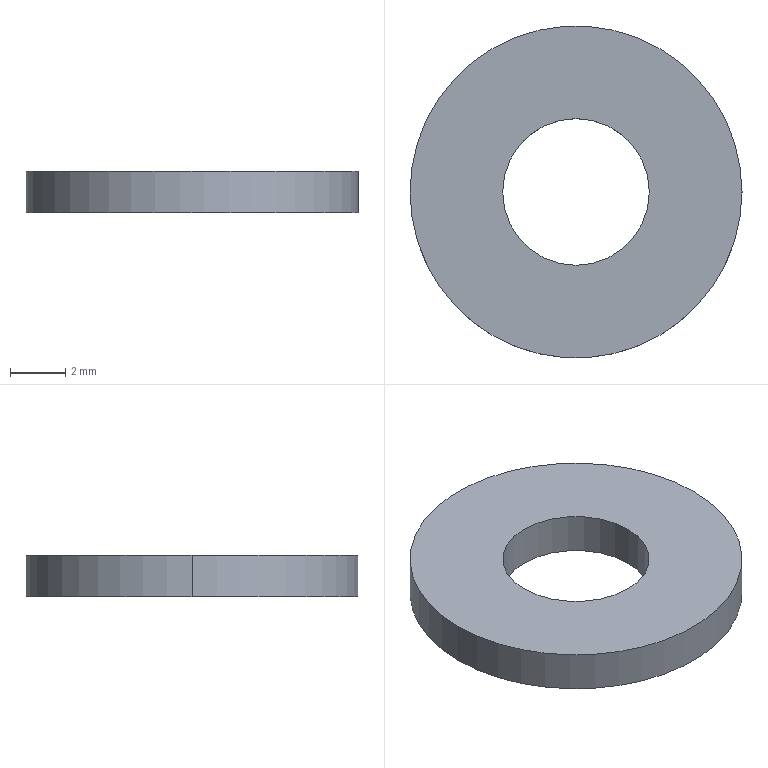Part | SolidWorks | features BaseBody 1 | 1 solid | 26 faces | box 12.059 x 12.059 x 1.507 mm | volume 122.712 mm3 | plane 14 | cylinder 12 | commonest cylinder face diameters 7.336 x4 10.049 x4 5.326 x2 12.059 x2
STEP:
#1=CARTESIAN_POINT('',(19.606,26.12,-12.71));
#2=VERTEX_POINT('',#1);
#3=CARTESIAN_POINT('',(7.547,26.12,-12.71));
#4=VERTEX_POINT('',#3);
#5=CARTESIAN_POINT('',(13.577,26.12,-12.71));
#6=DIRECTION('',(0.,0.,1.));
#7=DIRECTION('',(-1.,0.,0.));
#8=AXIS2_PLACEMENT_3D('',#5,#6,#7);
#9=CIRCLE('',#8,6.03);
#10=EDGE_CURVE('',#2,#4,#9,.T.);
#11=ORIENTED_EDGE('',*,*,#10,.F.);
#12=CARTESIAN_POINT('',(19.606,26.12,-14.217));
#13=VERTEX_POINT('',#12);
#14=CARTESIAN_POINT('',(19.606,26.12,-12.71));
#15=DIRECTION('',(0.,0.,-1.));
#16=VECTOR('',#15,1000.);
#17=LINE('',#14,#16);
#18=EDGE_CURVE('',#2,#13,#17,.T.);
#19=ORIENTED_EDGE('',*,*,#18,.T.);
#20=CARTESIAN_POINT('',(7.547,26.12,-14.217));
#21=VERTEX_POINT('',#20);
#22=CARTESIAN_POINT('',(13.577,26.12,-14.217));
#23=DIRECTION('',(0.,0.,1.));
#24=DIRECTION('',(-1.,0.,0.));
#25=AXIS2_PLACEMENT_3D('',#22,#23,#24);
#26=CIRCLE('',#25,6.03);
#27=EDGE_CURVE('',#13,#21,#26,.T.);
#28=ORIENTED_EDGE('',*,*,#27,.T.);
#29=CARTESIAN_POINT('',(7.547,26.12,-12.71));
#30=DIRECTION('',(0.,0.,-1.));
#31=VECTOR('',#30,1000.);
#32=LINE('',#29,#31);
#33=EDGE_CURVE('',#4,#21,#32,.T.);
#34=ORIENTED_EDGE('',*,*,#33,.F.);
#35=EDGE_LOOP('',(#11,#19,#28,#34));
#36=FACE_OUTER_BOUND('',#35,.T.);
#37=CARTESIAN_POINT('',(13.577,26.12,-12.71));
#38=DIRECTION('',(0.,0.,-1.));
#39=DIRECTION('',(-1.,0.,0.));
#40=AXIS2_PLACEMENT_3D('',#37,#38,#39);
#41=CYLINDRICAL_SURFACE('',#40,6.03);
#42=ADVANCED_FACE('',(#36),#41,.T.);
#43=CARTESIAN_POINT('',(16.24,26.12,-12.71));
#44=VERTEX_POINT('',#43);
#45=CARTESIAN_POINT('',(10.914,26.12,-12.71));
#46=VERTEX_POINT('',#45);
#47=CARTESIAN_POINT('',(13.577,26.12,-12.71));
#48=DIRECTION('',(0.,0.,-1.));
#49=DIRECTION('',(-1.,0.,0.));
#50=AXIS2_PLACEMENT_3D('',#47,#48,#49);
#51=CIRCLE('',#50,2.663);
#52=EDGE_CURVE('',#44,#46,#51,.T.);
#53=ORIENTED_EDGE('',*,*,#52,.F.);
#54=CARTESIAN_POINT('',(16.24,26.12,-14.217));
#55=VERTEX_POINT('',#54);
#56=CARTESIAN_POINT('',(16.24,26.12,-12.71));
#57=DIRECTION('',(0.,0.,-1.));
#58=VECTOR('',#57,1000.);
#59=LINE('',#56,#58);
#60=EDGE_CURVE('',#44,#55,#59,.T.);
#61=ORIENTED_EDGE('',*,*,#60,.T.);
#62=CARTESIAN_POINT('',(10.914,26.12,-14.217));
#63=VERTEX_POINT('',#62);
#64=CARTESIAN_POINT('',(13.577,26.12,-14.217));
#65=DIRECTION('',(0.,0.,1.));
#66=DIRECTION('',(-1.,0.,0.));
#67=AXIS2_PLACEMENT_3D('',#64,#65,#66);
#68=CIRCLE('',#67,2.663);
#69=EDGE_CURVE('',#63,#55,#68,.T.);
#70=ORIENTED_EDGE('',*,*,#69,.F.);
#71=CARTESIAN_POINT('',(10.914,26.12,-12.71));
#72=DIRECTION('',(0.,0.,-1.));
#73=VECTOR('',#72,1000.);
#74=LINE('',#71,#73);
#75=EDGE_CURVE('',#46,#63,#74,.T.);
#76=ORIENTED_EDGE('',*,*,#75,.F.);
#77=EDGE_LOOP('',(#53,#61,#70,#76));
#78=FACE_OUTER_BOUND('',#77,.T.);
#79=CARTESIAN_POINT('',(13.577,26.12,-12.71));
#80=DIRECTION('',(0.,0.,-1.));
#81=DIRECTION('',(-1.,0.,0.));
#82=AXIS2_PLACEMENT_3D('',#79,#80,#81);
#83=CYLINDRICAL_SURFACE('',#82,2.663);
#84=ADVANCED_FACE('',(#78),#83,.F.);
#85=CARTESIAN_POINT('',(13.577,26.12,-12.71));
#86=DIRECTION('',(0.,0.,1.));
#87=DIRECTION('',(-1.,0.,0.));
#88=AXIS2_PLACEMENT_3D('',#85,#86,#87);
#89=CIRCLE('',#88,6.03);
#90=EDGE_CURVE('',#4,#2,#89,.T.);
#91=ORIENTED_EDGE('',*,*,#90,.T.);
#92=ORIENTED_EDGE('',*,*,#10,.T.);
#93=EDGE_LOOP('',(#91,#92));
#94=FACE_OUTER_BOUND('',#93,.T.);
#95=CARTESIAN_POINT('',(13.577,26.12,-12.71));
#96=DIRECTION('',(0.,0.,-1.));
#97=DIRECTION('',(-1.,0.,0.));
#98=AXIS2_PLACEMENT_3D('',#95,#96,#97);
#99=CIRCLE('',#98,2.663);
#100=EDGE_CURVE('',#46,#44,#99,.T.);
#101=ORIENTED_EDGE('',*,*,#100,.T.);
#102=ORIENTED_EDGE('',*,*,#52,.T.);
#103=EDGE_LOOP('',(#101,#102));
#104=FACE_BOUND('',#103,.T.);
#105=CARTESIAN_POINT('',(13.577,26.12,-12.71));
#106=DIRECTION('',(0.,0.,1.));
#107=DIRECTION('',(1.,0.,0.));
#108=AXIS2_PLACEMENT_3D('',#105,#106,#107);
#109=PLANE('',#108);
#110=ADVANCED_FACE('',(#94,#104),#109,.T.);
#111=ORIENTED_EDGE('',*,*,#18,.F.);
#112=ORIENTED_EDGE('',*,*,#90,.F.);
#113=ORIENTED_EDGE('',*,*,#33,.T.);
#114=CARTESIAN_POINT('',(13.577,26.12,-14.217));
#115=DIRECTION('',(0.,0.,1.));
#116=DIRECTION('',(-1.,0.,0.));
#117=AXIS2_PLACEMENT_3D('',#114,#115,#116);
#118=CIRCLE('',#117,6.03);
#119=EDGE_CURVE('',#21,#13,#118,.T.);
#120=ORIENTED_EDGE('',*,*,#119,.T.);
#121=EDGE_LOOP('',(#111,#112,#113,#120));
#122=FACE_OUTER_BOUND('',#121,.T.);
#123=CARTESIAN_POINT('',(13.577,26.12,-12.71));
#124=DIRECTION('',(0.,0.,-1.));
#125=DIRECTION('',(-1.,0.,0.));
#126=AXIS2_PLACEMENT_3D('',#123,#124,#125);
#127=CYLINDRICAL_SURFACE('',#126,6.03);
#128=ADVANCED_FACE('',(#122),#127,.T.);
#129=ORIENTED_EDGE('',*,*,#60,.F.);
#130=ORIENTED_EDGE('',*,*,#100,.F.);
#131=ORIENTED_EDGE('',*,*,#75,.T.);
#132=CARTESIAN_POINT('',(13.577,26.12,-14.217));
#133=DIRECTION('',(0.,0.,1.));
#134=DIRECTION('',(-1.,0.,0.));
#135=AXIS2_PLACEMENT_3D('',#132,#133,#134);
#136=CIRCLE('',#135,2.663);
#137=EDGE_CURVE('',#55,#63,#136,.T.);
#138=ORIENTED_EDGE('',*,*,#137,.F.);
#139=EDGE_LOOP('',(#129,#130,#131,#138));
#140=FACE_OUTER_BOUND('',#139,.T.);
#141=CARTESIAN_POINT('',(13.577,26.12,-12.71));
#142=DIRECTION('',(0.,0.,-1.));
#143=DIRECTION('',(-1.,0.,0.));
#144=AXIS2_PLACEMENT_3D('',#141,#142,#143);
#145=CYLINDRICAL_SURFACE('',#144,2.663);
#146=ADVANCED_FACE('',(#140),#145,.F.);
#147=CARTESIAN_POINT('',(18.576,25.618,-14.217));
#148=VERTEX_POINT('',#147);
#149=CARTESIAN_POINT('',(14.079,21.121,-14.217));
#150=VERTEX_POINT('',#149);
#151=CARTESIAN_POINT('',(13.577,26.12,-14.217));
#152=DIRECTION('',(0.,0.,-1.));
#153=DIRECTION('',(-1.,0.,0.));
#154=AXIS2_PLACEMENT_3D('',#151,#152,#153);
#155=CIRCLE('',#154,5.025);
#156=EDGE_CURVE('',#148,#150,#155,.T.);
#157=ORIENTED_EDGE('',*,*,#156,.F.);
#158=CARTESIAN_POINT('',(17.21,25.618,-14.217));
#159=VERTEX_POINT('',#158);
#160=CARTESIAN_POINT('',(13.577,25.618,-14.217));
#161=DIRECTION('',(1.,0.,0.));
#162=VECTOR('',#161,1000.);
#163=LINE('',#160,#162);
#164=EDGE_CURVE('',#159,#148,#163,.T.);
#165=ORIENTED_EDGE('',*,*,#164,.F.);
#166=CARTESIAN_POINT('',(14.079,22.487,-14.217));
#167=VERTEX_POINT('',#166);
#168=CARTESIAN_POINT('',(13.577,26.12,-14.217));
#169=DIRECTION('',(0.,0.,1.));
#170=DIRECTION('',(-1.,0.,0.));
#171=AXIS2_PLACEMENT_3D('',#168,#169,#170);
#172=CIRCLE('',#171,3.668);
#173=EDGE_CURVE('',#167,#159,#172,.T.);
#174=ORIENTED_EDGE('',*,*,#173,.F.);
#175=CARTESIAN_POINT('',(14.079,26.12,-14.217));
#176=DIRECTION('',(0.,1.,0.));
#177=VECTOR('',#176,1000.);
#178=LINE('',#175,#177);
#179=EDGE_CURVE('',#150,#167,#178,.T.);
#180=ORIENTED_EDGE('',*,*,#179,.F.);
#181=EDGE_LOOP('',(#157,#165,#174,#180));
#182=FACE_BOUND('',#181,.T.);
#183=CARTESIAN_POINT('',(13.074,22.487,-14.217));
#184=VERTEX_POINT('',#183);
#185=CARTESIAN_POINT('',(13.074,21.121,-14.217));
#186=VERTEX_POINT('',#185);
#187=CARTESIAN_POINT('',(13.074,26.12,-14.217));
#188=DIRECTION('',(0.,-1.,0.));
#189=VECTOR('',#188,1000.);
#190=LINE('',#187,#189);
#191=EDGE_CURVE('',#184,#186,#190,.T.);
#192=ORIENTED_EDGE('',*,*,#191,.F.);
#193=CARTESIAN_POINT('',(9.943,25.618,-14.217));
#194=VERTEX_POINT('',#193);
#195=CARTESIAN_POINT('',(13.577,26.12,-14.217));
#196=DIRECTION('',(0.,0.,1.));
#197=DIRECTION('',(-1.,0.,0.));
#198=AXIS2_PLACEMENT_3D('',#195,#196,#197);
#199=CIRCLE('',#198,3.668);
#200=EDGE_CURVE('',#194,#184,#199,.T.);
#201=ORIENTED_EDGE('',*,*,#200,.F.);
#202=CARTESIAN_POINT('',(8.577,25.618,-14.217));
#203=VERTEX_POINT('',#202);
#204=CARTESIAN_POINT('',(13.577,25.618,-14.217));
#205=DIRECTION('',(1.,0.,0.));
#206=VECTOR('',#205,1000.);
#207=LINE('',#204,#206);
#208=EDGE_CURVE('',#203,#194,#207,.T.);
#209=ORIENTED_EDGE('',*,*,#208,.F.);
#210=CARTESIAN_POINT('',(13.577,26.12,-14.217));
#211=DIRECTION('',(0.,0.,-1.));
#212=DIRECTION('',(-1.,0.,0.));
#213=AXIS2_PLACEMENT_3D('',#210,#211,#212);
#214=CIRCLE('',#213,5.025);
#215=EDGE_CURVE('',#186,#203,#214,.T.);
#216=ORIENTED_EDGE('',*,*,#215,.F.);
#217=EDGE_LOOP('',(#192,#201,#209,#216));
#218=FACE_BOUND('',#217,.T.);
#219=ORIENTED_EDGE('',*,*,#119,.F.);
#220=ORIENTED_EDGE('',*,*,#27,.F.);
#221=EDGE_LOOP('',(#219,#220));
#222=FACE_OUTER_BOUND('',#221,.T.);
#223=CARTESIAN_POINT('',(14.079,29.753,-14.217));
#224=VERTEX_POINT('',#223);
#225=CARTESIAN_POINT('',(14.079,31.119,-14.217));
#226=VERTEX_POINT('',#225);
#227=CARTESIAN_POINT('',(14.079,26.12,-14.217));
#228=DIRECTION('',(0.,1.,0.));
#229=VECTOR('',#228,1000.);
#230=LINE('',#227,#229);
#231=EDGE_CURVE('',#224,#226,#230,.T.);
#232=ORIENTED_EDGE('',*,*,#231,.F.);
#233=CARTESIAN_POINT('',(17.21,26.622,-14.217));
#234=VERTEX_POINT('',#233);
#235=CARTESIAN_POINT('',(13.577,26.12,-14.217));
#236=DIRECTION('',(0.,0.,1.));
#237=DIRECTION('',(-1.,0.,0.));
#238=AXIS2_PLACEMENT_3D('',#235,#236,#237);
#239=CIRCLE('',#238,3.668);
#240=EDGE_CURVE('',#234,#224,#239,.T.);
#241=ORIENTED_EDGE('',*,*,#240,.F.);
#242=CARTESIAN_POINT('',(18.576,26.622,-14.217));
#243=VERTEX_POINT('',#242);
#244=CARTESIAN_POINT('',(13.577,26.622,-14.217));
#245=DIRECTION('',(-1.,0.,0.));
#246=VECTOR('',#245,1000.);
#247=LINE('',#244,#246);
#248=EDGE_CURVE('',#243,#234,#247,.T.);
#249=ORIENTED_EDGE('',*,*,#248,.F.);
#250=CARTESIAN_POINT('',(13.577,26.12,-14.217));
#251=DIRECTION('',(0.,0.,-1.));
#252=DIRECTION('',(-1.,0.,0.));
#253=AXIS2_PLACEMENT_3D('',#250,#251,#252);
#254=CIRCLE('',#253,5.025);
#255=EDGE_CURVE('',#226,#243,#254,.T.);
#256=ORIENTED_EDGE('',*,*,#255,.F.);
#257=EDGE_LOOP('',(#232,#241,#249,#256));
#258=FACE_BOUND('',#257,.T.);
#259=ORIENTED_EDGE('',*,*,#69,.T.);
#260=ORIENTED_EDGE('',*,*,#137,.T.);
#261=EDGE_LOOP('',(#259,#260));
#262=FACE_BOUND('',#261,.T.);
#263=CARTESIAN_POINT('',(8.577,26.622,-14.217));
#264=VERTEX_POINT('',#263);
#265=CARTESIAN_POINT('',(13.074,31.119,-14.217));
#266=VERTEX_POINT('',#265);
#267=CARTESIAN_POINT('',(13.577,26.12,-14.217));
#268=DIRECTION('',(0.,0.,-1.));
#269=DIRECTION('',(-1.,0.,0.));
#270=AXIS2_PLACEMENT_3D('',#267,#268,#269);
#271=CIRCLE('',#270,5.025);
#272=EDGE_CURVE('',#264,#266,#271,.T.);
#273=ORIENTED_EDGE('',*,*,#272,.F.);
#274=CARTESIAN_POINT('',(9.943,26.622,-14.217));
#275=VERTEX_POINT('',#274);
#276=CARTESIAN_POINT('',(13.577,26.622,-14.217));
#277=DIRECTION('',(-1.,0.,0.));
#278=VECTOR('',#277,1000.);
#279=LINE('',#276,#278);
#280=EDGE_CURVE('',#275,#264,#279,.T.);
#281=ORIENTED_EDGE('',*,*,#280,.F.);
#282=CARTESIAN_POINT('',(13.074,29.753,-14.217));
#283=VERTEX_POINT('',#282);
#284=CARTESIAN_POINT('',(13.577,26.12,-14.217));
#285=DIRECTION('',(0.,0.,1.));
#286=DIRECTION('',(-1.,0.,0.));
#287=AXIS2_PLACEMENT_3D('',#284,#285,#286);
#288=CIRCLE('',#287,3.668);
#289=EDGE_CURVE('',#283,#275,#288,.T.);
#290=ORIENTED_EDGE('',*,*,#289,.F.);
#291=CARTESIAN_POINT('',(13.074,26.12,-14.217));
#292=DIRECTION('',(0.,-1.,0.));
#293=VECTOR('',#292,1000.);
#294=LINE('',#291,#293);
#295=EDGE_CURVE('',#266,#283,#294,.T.);
#296=ORIENTED_EDGE('',*,*,#295,.F.);
#297=EDGE_LOOP('',(#273,#281,#290,#296));
#298=FACE_BOUND('',#297,.T.);
#299=CARTESIAN_POINT('',(13.577,26.12,-14.217));
#300=DIRECTION('',(0.,0.,1.));
#301=DIRECTION('',(1.,0.,0.));
#302=AXIS2_PLACEMENT_3D('',#299,#300,#301);
#303=PLANE('',#302);
#304=ADVANCED_FACE('',(#182,#218,#222,#258,#262,#298),#303,.F.);
#305=CARTESIAN_POINT('',(14.079,22.487,-13.715));
#306=VERTEX_POINT('',#305);
#307=CARTESIAN_POINT('',(14.079,21.121,-13.715));
#308=VERTEX_POINT('',#307);
#309=CARTESIAN_POINT('',(14.079,26.12,-13.715));
#310=DIRECTION('',(0.,-1.,0.));
#311=VECTOR('',#310,1000.);
#312=LINE('',#309,#311);
#313=EDGE_CURVE('',#306,#308,#312,.T.);
#314=ORIENTED_EDGE('',*,*,#313,.T.);
#315=CARTESIAN_POINT('',(14.079,21.121,-14.217));
#316=DIRECTION('',(0.,0.,1.));
#317=VECTOR('',#316,1000.);
#318=LINE('',#315,#317);
#319=EDGE_CURVE('',#150,#308,#318,.T.);
#320=ORIENTED_EDGE('',*,*,#319,.F.);
#321=ORIENTED_EDGE('',*,*,#179,.T.);
#322=CARTESIAN_POINT('',(14.079,22.487,-14.217));
#323=DIRECTION('',(0.,0.,-1.));
#324=VECTOR('',#323,1000.);
#325=LINE('',#322,#324);
#326=EDGE_CURVE('',#306,#167,#325,.T.);
#327=ORIENTED_EDGE('',*,*,#326,.F.);
#328=EDGE_LOOP('',(#314,#320,#321,#327));
#329=FACE_OUTER_BOUND('',#328,.T.);
#330=CARTESIAN_POINT('',(14.079,22.882,-14.217));
#331=DIRECTION('',(-1.,0.,0.));
#332=DIRECTION('',(0.,-1.,0.));
#333=AXIS2_PLACEMENT_3D('',#330,#331,#332);
#334=PLANE('',#333);
#335=ADVANCED_FACE('',(#329),#334,.F.);
#336=CARTESIAN_POINT('',(18.576,25.618,-13.715));
#337=VERTEX_POINT('',#336);
#338=CARTESIAN_POINT('',(18.576,25.618,-12.71));
#339=DIRECTION('',(0.,0.,1.));
#340=VECTOR('',#339,1000.);
#341=LINE('',#338,#340);
#342=EDGE_CURVE('',#148,#337,#341,.T.);
#343=ORIENTED_EDGE('',*,*,#342,.F.);
#344=ORIENTED_EDGE('',*,*,#156,.T.);
#345=ORIENTED_EDGE('',*,*,#319,.T.);
#346=CARTESIAN_POINT('',(13.577,26.12,-13.715));
#347=DIRECTION('',(0.,0.,-1.));
#348=DIRECTION('',(-1.,0.,0.));
#349=AXIS2_PLACEMENT_3D('',#346,#347,#348);
#350=CIRCLE('',#349,5.025);
#351=EDGE_CURVE('',#337,#308,#350,.T.);
#352=ORIENTED_EDGE('',*,*,#351,.F.);
#353=EDGE_LOOP('',(#343,#344,#345,#352));
#354=FACE_OUTER_BOUND('',#353,.T.);
#355=CARTESIAN_POINT('',(13.577,26.12,-12.71));
#356=DIRECTION('',(0.,0.,-1.));
#357=DIRECTION('',(-1.,0.,0.));
#358=AXIS2_PLACEMENT_3D('',#355,#356,#357);
#359=CYLINDRICAL_SURFACE('',#358,5.025);
#360=ADVANCED_FACE('',(#354),#359,.F.);
#361=CARTESIAN_POINT('',(17.21,25.618,-13.715));
#362=VERTEX_POINT('',#361);
#363=CARTESIAN_POINT('',(16.815,25.618,-13.715));
#364=DIRECTION('',(-1.,0.,0.));
#365=VECTOR('',#364,1000.);
#366=LINE('',#363,#365);
#367=EDGE_CURVE('',#337,#362,#366,.T.);
#368=ORIENTED_EDGE('',*,*,#367,.T.);
#369=CARTESIAN_POINT('',(17.21,25.618,-14.217));
#370=DIRECTION('',(0.,0.,-1.));
#371=VECTOR('',#370,1000.);
#372=LINE('',#369,#371);
#373=EDGE_CURVE('',#362,#159,#372,.T.);
#374=ORIENTED_EDGE('',*,*,#373,.T.);
#375=ORIENTED_EDGE('',*,*,#164,.T.);
#376=ORIENTED_EDGE('',*,*,#342,.T.);
#377=EDGE_LOOP('',(#368,#374,#375,#376));
#378=FACE_OUTER_BOUND('',#377,.T.);
#379=CARTESIAN_POINT('',(16.815,25.618,-14.217));
#380=DIRECTION('',(0.,-1.,0.));
#381=DIRECTION('',(1.,0.,0.));
#382=AXIS2_PLACEMENT_3D('',#379,#380,#381);
#383=PLANE('',#382);
#384=ADVANCED_FACE('',(#378),#383,.T.);
#385=ORIENTED_EDGE('',*,*,#373,.F.);
#386=CARTESIAN_POINT('',(13.577,26.12,-13.715));
#387=DIRECTION('',(0.,0.,-1.));
#388=DIRECTION('',(-1.,0.,0.));
#389=AXIS2_PLACEMENT_3D('',#386,#387,#388);
#390=CIRCLE('',#389,3.668);
#391=EDGE_CURVE('',#362,#306,#390,.T.);
#392=ORIENTED_EDGE('',*,*,#391,.T.);
#393=ORIENTED_EDGE('',*,*,#326,.T.);
#394=ORIENTED_EDGE('',*,*,#173,.T.);
#395=EDGE_LOOP('',(#385,#392,#393,#394));
#396=FACE_OUTER_BOUND('',#395,.T.);
#397=CARTESIAN_POINT('',(13.577,26.12,-12.71));
#398=DIRECTION('',(0.,0.,-1.));
#399=DIRECTION('',(-1.,0.,0.));
#400=AXIS2_PLACEMENT_3D('',#397,#398,#399);
#401=CYLINDRICAL_SURFACE('',#400,3.668);
#402=ADVANCED_FACE('',(#396),#401,.T.);
#403=CARTESIAN_POINT('',(13.074,21.121,-13.715));
#404=VERTEX_POINT('',#403);
#405=CARTESIAN_POINT('',(13.074,21.121,-12.71));
#406=DIRECTION('',(0.,0.,1.));
#407=VECTOR('',#406,1000.);
#408=LINE('',#405,#407);
#409=EDGE_CURVE('',#186,#404,#408,.T.);
#410=ORIENTED_EDGE('',*,*,#409,.F.);
#411=ORIENTED_EDGE('',*,*,#215,.T.);
#412=CARTESIAN_POINT('',(8.577,25.618,-13.715));
#413=VERTEX_POINT('',#412);
#414=CARTESIAN_POINT('',(8.577,25.618,-12.71));
#415=DIRECTION('',(0.,0.,-1.));
#416=VECTOR('',#415,1000.);
#417=LINE('',#414,#416);
#418=EDGE_CURVE('',#413,#203,#417,.T.);
#419=ORIENTED_EDGE('',*,*,#418,.F.);
#420=CARTESIAN_POINT('',(13.577,26.12,-13.715));
#421=DIRECTION('',(0.,0.,-1.));
#422=DIRECTION('',(-1.,0.,0.));
#423=AXIS2_PLACEMENT_3D('',#420,#421,#422);
#424=CIRCLE('',#423,5.025);
#425=EDGE_CURVE('',#404,#413,#424,.T.);
#426=ORIENTED_EDGE('',*,*,#425,.F.);
#427=EDGE_LOOP('',(#410,#411,#419,#426));
#428=FACE_OUTER_BOUND('',#427,.T.);
#429=CARTESIAN_POINT('',(13.577,26.12,-12.71));
#430=DIRECTION('',(0.,0.,-1.));
#431=DIRECTION('',(-1.,0.,0.));
#432=AXIS2_PLACEMENT_3D('',#429,#430,#431);
#433=CYLINDRICAL_SURFACE('',#432,5.025);
#434=ADVANCED_FACE('',(#428),#433,.F.);
#435=CARTESIAN_POINT('',(13.074,22.487,-13.715));
#436=VERTEX_POINT('',#435);
#437=CARTESIAN_POINT('',(13.074,22.882,-13.715));
#438=DIRECTION('',(0.,1.,0.));
#439=VECTOR('',#438,1000.);
#440=LINE('',#437,#439);
#441=EDGE_CURVE('',#404,#436,#440,.T.);
#442=ORIENTED_EDGE('',*,*,#441,.T.);
#443=CARTESIAN_POINT('',(13.074,22.487,-14.217));
#444=DIRECTION('',(0.,0.,-1.));
#445=VECTOR('',#444,1000.);
#446=LINE('',#443,#445);
#447=EDGE_CURVE('',#436,#184,#446,.T.);
#448=ORIENTED_EDGE('',*,*,#447,.T.);
#449=ORIENTED_EDGE('',*,*,#191,.T.);
#450=ORIENTED_EDGE('',*,*,#409,.T.);
#451=EDGE_LOOP('',(#442,#448,#449,#450));
#452=FACE_OUTER_BOUND('',#451,.T.);
#453=CARTESIAN_POINT('',(13.074,22.882,-14.217));
#454=DIRECTION('',(-1.,0.,0.));
#455=DIRECTION('',(0.,-1.,0.));
#456=AXIS2_PLACEMENT_3D('',#453,#454,#455);
#457=PLANE('',#456);
#458=ADVANCED_FACE('',(#452),#457,.T.);
#459=ORIENTED_EDGE('',*,*,#447,.F.);
#460=CARTESIAN_POINT('',(9.943,25.618,-13.715));
#461=VERTEX_POINT('',#460);
#462=CARTESIAN_POINT('',(13.577,26.12,-13.715));
#463=DIRECTION('',(0.,0.,-1.));
#464=DIRECTION('',(-1.,0.,0.));
#465=AXIS2_PLACEMENT_3D('',#462,#463,#464);
#466=CIRCLE('',#465,3.668);
#467=EDGE_CURVE('',#436,#461,#466,.T.);
#468=ORIENTED_EDGE('',*,*,#467,.T.);
#469=CARTESIAN_POINT('',(9.943,25.618,-12.71));
#470=DIRECTION('',(0.,0.,-1.));
#471=VECTOR('',#470,1000.);
#472=LINE('',#469,#471);
#473=EDGE_CURVE('',#461,#194,#472,.T.);
#474=ORIENTED_EDGE('',*,*,#473,.T.);
#475=ORIENTED_EDGE('',*,*,#200,.T.);
#476=EDGE_LOOP('',(#459,#468,#474,#475));
#477=FACE_OUTER_BOUND('',#476,.T.);
#478=CARTESIAN_POINT('',(13.577,26.12,-12.71));
#479=DIRECTION('',(0.,0.,-1.));
#480=DIRECTION('',(-1.,0.,0.));
#481=AXIS2_PLACEMENT_3D('',#478,#479,#480);
#482=CYLINDRICAL_SURFACE('',#481,3.668);
#483=ADVANCED_FACE('',(#477),#482,.T.);
#484=CARTESIAN_POINT('',(10.338,25.618,-13.715));
#485=DIRECTION('',(1.,0.,0.));
#486=VECTOR('',#485,1000.);
#487=LINE('',#484,#486);
#488=EDGE_CURVE('',#413,#461,#487,.T.);
#489=ORIENTED_EDGE('',*,*,#488,.F.);
#490=ORIENTED_EDGE('',*,*,#418,.T.);
#491=ORIENTED_EDGE('',*,*,#208,.T.);
#492=ORIENTED_EDGE('',*,*,#473,.F.);
#493=EDGE_LOOP('',(#489,#490,#491,#492));
#494=FACE_OUTER_BOUND('',#493,.T.);
#495=CARTESIAN_POINT('',(10.338,25.618,-14.217));
#496=DIRECTION('',(0.,1.,0.));
#497=DIRECTION('',(-1.,0.,0.));
#498=AXIS2_PLACEMENT_3D('',#495,#496,#497);
#499=PLANE('',#498);
#500=ADVANCED_FACE('',(#494),#499,.F.);
#501=CARTESIAN_POINT('',(14.079,31.119,-13.715));
#502=VERTEX_POINT('',#501);
#503=CARTESIAN_POINT('',(14.079,31.119,-12.71));
#504=DIRECTION('',(0.,0.,1.));
#505=VECTOR('',#504,1000.);
#506=LINE('',#503,#505);
#507=EDGE_CURVE('',#226,#502,#506,.T.);
#508=ORIENTED_EDGE('',*,*,#507,.F.);
#509=ORIENTED_EDGE('',*,*,#255,.T.);
#510=CARTESIAN_POINT('',(18.576,26.622,-13.715));
#511=VERTEX_POINT('',#510);
#512=CARTESIAN_POINT('',(18.576,26.622,-12.71));
#513=DIRECTION('',(0.,0.,-1.));
#514=VECTOR('',#513,1000.);
#515=LINE('',#512,#514);
#516=EDGE_CURVE('',#511,#243,#515,.T.);
#517=ORIENTED_EDGE('',*,*,#516,.F.);
#518=CARTESIAN_POINT('',(13.577,26.12,-13.715));
#519=DIRECTION('',(0.,0.,-1.));
#520=DIRECTION('',(-1.,0.,0.));
#521=AXIS2_PLACEMENT_3D('',#518,#519,#520);
#522=CIRCLE('',#521,5.025);
#523=EDGE_CURVE('',#502,#511,#522,.T.);
#524=ORIENTED_EDGE('',*,*,#523,.F.);
#525=EDGE_LOOP('',(#508,#509,#517,#524));
#526=FACE_OUTER_BOUND('',#525,.T.);
#527=CARTESIAN_POINT('',(13.577,26.12,-12.71));
#528=DIRECTION('',(0.,0.,-1.));
#529=DIRECTION('',(-1.,0.,0.));
#530=AXIS2_PLACEMENT_3D('',#527,#528,#529);
#531=CYLINDRICAL_SURFACE('',#530,5.025);
#532=ADVANCED_FACE('',(#526),#531,.F.);
#533=CARTESIAN_POINT('',(14.079,29.753,-13.715));
#534=VERTEX_POINT('',#533);
#535=CARTESIAN_POINT('',(14.079,29.358,-13.715));
#536=DIRECTION('',(0.,-1.,0.));
#537=VECTOR('',#536,1000.);
#538=LINE('',#535,#537);
#539=EDGE_CURVE('',#502,#534,#538,.T.);
#540=ORIENTED_EDGE('',*,*,#539,.T.);
#541=CARTESIAN_POINT('',(14.079,29.753,-14.217));
#542=DIRECTION('',(0.,0.,-1.));
#543=VECTOR('',#542,1000.);
#544=LINE('',#541,#543);
#545=EDGE_CURVE('',#534,#224,#544,.T.);
#546=ORIENTED_EDGE('',*,*,#545,.T.);
#547=ORIENTED_EDGE('',*,*,#231,.T.);
#548=ORIENTED_EDGE('',*,*,#507,.T.);
#549=EDGE_LOOP('',(#540,#546,#547,#548));
#550=FACE_OUTER_BOUND('',#549,.T.);
#551=CARTESIAN_POINT('',(14.079,29.358,-14.217));
#552=DIRECTION('',(1.,0.,0.));
#553=DIRECTION('',(0.,1.,0.));
#554=AXIS2_PLACEMENT_3D('',#551,#552,#553);
#555=PLANE('',#554);
#556=ADVANCED_FACE('',(#550),#555,.T.);
#557=ORIENTED_EDGE('',*,*,#545,.F.);
#558=CARTESIAN_POINT('',(17.21,26.622,-13.715));
#559=VERTEX_POINT('',#558);
#560=CARTESIAN_POINT('',(13.577,26.12,-13.715));
#561=DIRECTION('',(0.,0.,-1.));
#562=DIRECTION('',(-1.,0.,0.));
#563=AXIS2_PLACEMENT_3D('',#560,#561,#562);
#564=CIRCLE('',#563,3.668);
#565=EDGE_CURVE('',#534,#559,#564,.T.);
#566=ORIENTED_EDGE('',*,*,#565,.T.);
#567=CARTESIAN_POINT('',(17.21,26.622,-12.71));
#568=DIRECTION('',(0.,0.,-1.));
#569=VECTOR('',#568,1000.);
#570=LINE('',#567,#569);
#571=EDGE_CURVE('',#559,#234,#570,.T.);
#572=ORIENTED_EDGE('',*,*,#571,.T.);
#573=ORIENTED_EDGE('',*,*,#240,.T.);
#574=EDGE_LOOP('',(#557,#566,#572,#573));
#575=FACE_OUTER_BOUND('',#574,.T.);
#576=CARTESIAN_POINT('',(13.577,26.12,-12.71));
#577=DIRECTION('',(0.,0.,-1.));
#578=DIRECTION('',(-1.,0.,0.));
#579=AXIS2_PLACEMENT_3D('',#576,#577,#578);
#580=CYLINDRICAL_SURFACE('',#579,3.668);
#581=ADVANCED_FACE('',(#575),#580,.T.);
#582=CARTESIAN_POINT('',(16.815,26.622,-13.715));
#583=DIRECTION('',(-1.,0.,0.));
#584=VECTOR('',#583,1000.);
#585=LINE('',#582,#584);
#586=EDGE_CURVE('',#511,#559,#585,.T.);
#587=ORIENTED_EDGE('',*,*,#586,.F.);
#588=ORIENTED_EDGE('',*,*,#516,.T.);
#589=ORIENTED_EDGE('',*,*,#248,.T.);
#590=ORIENTED_EDGE('',*,*,#571,.F.);
#591=EDGE_LOOP('',(#587,#588,#589,#590));
#592=FACE_OUTER_BOUND('',#591,.T.);
#593=CARTESIAN_POINT('',(16.815,26.622,-14.217));
#594=DIRECTION('',(0.,-1.,0.));
#595=DIRECTION('',(1.,0.,0.));
#596=AXIS2_PLACEMENT_3D('',#593,#594,#595);
#597=PLANE('',#596);
#598=ADVANCED_FACE('',(#592),#597,.F.);
#599=CARTESIAN_POINT('',(13.074,29.753,-13.715));
#600=VERTEX_POINT('',#599);
#601=CARTESIAN_POINT('',(13.074,31.119,-13.715));
#602=VERTEX_POINT('',#601);
#603=CARTESIAN_POINT('',(13.074,26.12,-13.715));
#604=DIRECTION('',(0.,1.,0.));
#605=VECTOR('',#604,1000.);
#606=LINE('',#603,#605);
#607=EDGE_CURVE('',#600,#602,#606,.T.);
#608=ORIENTED_EDGE('',*,*,#607,.T.);
#609=CARTESIAN_POINT('',(13.074,31.119,-14.217));
#610=DIRECTION('',(0.,0.,1.));
#611=VECTOR('',#610,1000.);
#612=LINE('',#609,#611);
#613=EDGE_CURVE('',#266,#602,#612,.T.);
#614=ORIENTED_EDGE('',*,*,#613,.F.);
#615=ORIENTED_EDGE('',*,*,#295,.T.);
#616=CARTESIAN_POINT('',(13.074,29.753,-14.217));
#617=DIRECTION('',(0.,0.,-1.));
#618=VECTOR('',#617,1000.);
#619=LINE('',#616,#618);
#620=EDGE_CURVE('',#600,#283,#619,.T.);
#621=ORIENTED_EDGE('',*,*,#620,.F.);
#622=EDGE_LOOP('',(#608,#614,#615,#621));
#623=FACE_OUTER_BOUND('',#622,.T.);
#624=CARTESIAN_POINT('',(13.074,29.358,-14.217));
#625=DIRECTION('',(1.,0.,0.));
#626=DIRECTION('',(0.,1.,0.));
#627=AXIS2_PLACEMENT_3D('',#624,#625,#626);
#628=PLANE('',#627);
#629=ADVANCED_FACE('',(#623),#628,.F.);
#630=CARTESIAN_POINT('',(8.577,26.622,-13.715));
#631=VERTEX_POINT('',#630);
#632=CARTESIAN_POINT('',(13.577,26.12,-13.715));
#633=DIRECTION('',(0.,0.,-1.));
#634=DIRECTION('',(-1.,0.,0.));
#635=AXIS2_PLACEMENT_3D('',#632,#633,#634);
#636=CIRCLE('',#635,5.025);
#637=EDGE_CURVE('',#631,#602,#636,.T.);
#638=ORIENTED_EDGE('',*,*,#637,.F.);
#639=CARTESIAN_POINT('',(8.577,26.622,-12.71));
#640=DIRECTION('',(0.,0.,1.));
#641=VECTOR('',#640,1000.);
#642=LINE('',#639,#641);
#643=EDGE_CURVE('',#264,#631,#642,.T.);
#644=ORIENTED_EDGE('',*,*,#643,.F.);
#645=ORIENTED_EDGE('',*,*,#272,.T.);
#646=ORIENTED_EDGE('',*,*,#613,.T.);
#647=EDGE_LOOP('',(#638,#644,#645,#646));
#648=FACE_OUTER_BOUND('',#647,.T.);
#649=CARTESIAN_POINT('',(13.577,26.12,-12.71));
#650=DIRECTION('',(0.,0.,-1.));
#651=DIRECTION('',(-1.,0.,0.));
#652=AXIS2_PLACEMENT_3D('',#649,#650,#651);
#653=CYLINDRICAL_SURFACE('',#652,5.025);
#654=ADVANCED_FACE('',(#648),#653,.F.);
#655=CARTESIAN_POINT('',(9.943,26.622,-13.715));
#656=VERTEX_POINT('',#655);
#657=CARTESIAN_POINT('',(10.338,26.622,-13.715));
#658=DIRECTION('',(1.,0.,0.));
#659=VECTOR('',#658,1000.);
#660=LINE('',#657,#659);
#661=EDGE_CURVE('',#631,#656,#660,.T.);
#662=ORIENTED_EDGE('',*,*,#661,.T.);
#663=CARTESIAN_POINT('',(9.943,26.622,-14.217));
#664=DIRECTION('',(0.,0.,-1.));
#665=VECTOR('',#664,1000.);
#666=LINE('',#663,#665);
#667=EDGE_CURVE('',#656,#275,#666,.T.);
#668=ORIENTED_EDGE('',*,*,#667,.T.);
#669=ORIENTED_EDGE('',*,*,#280,.T.);
#670=ORIENTED_EDGE('',*,*,#643,.T.);
#671=EDGE_LOOP('',(#662,#668,#669,#670));
#672=FACE_OUTER_BOUND('',#671,.T.);
#673=CARTESIAN_POINT('',(10.338,26.622,-14.217));
#674=DIRECTION('',(0.,1.,0.));
#675=DIRECTION('',(-1.,0.,0.));
#676=AXIS2_PLACEMENT_3D('',#673,#674,#675);
#677=PLANE('',#676);
#678=ADVANCED_FACE('',(#672),#677,.T.);
#679=CARTESIAN_POINT('',(13.577,26.12,-13.715));
#680=DIRECTION('',(0.,0.,-1.));
#681=DIRECTION('',(-1.,0.,0.));
#682=AXIS2_PLACEMENT_3D('',#679,#680,#681);
#683=CIRCLE('',#682,3.668);
#684=EDGE_CURVE('',#656,#600,#683,.T.);
#685=ORIENTED_EDGE('',*,*,#684,.T.);
#686=ORIENTED_EDGE('',*,*,#620,.T.);
#687=ORIENTED_EDGE('',*,*,#289,.T.);
#688=ORIENTED_EDGE('',*,*,#667,.F.);
#689=EDGE_LOOP('',(#685,#686,#687,#688));
#690=FACE_OUTER_BOUND('',#689,.T.);
#691=CARTESIAN_POINT('',(13.577,26.12,-12.71));
#692=DIRECTION('',(0.,0.,-1.));
#693=DIRECTION('',(-1.,0.,0.));
#694=AXIS2_PLACEMENT_3D('',#691,#692,#693);
#695=CYLINDRICAL_SURFACE('',#694,3.668);
#696=ADVANCED_FACE('',(#690),#695,.T.);
#697=ORIENTED_EDGE('',*,*,#351,.T.);
#698=ORIENTED_EDGE('',*,*,#313,.F.);
#699=ORIENTED_EDGE('',*,*,#391,.F.);
#700=ORIENTED_EDGE('',*,*,#367,.F.);
#701=EDGE_LOOP('',(#697,#698,#699,#700));
#702=FACE_OUTER_BOUND('',#701,.T.);
#703=CARTESIAN_POINT('',(13.577,26.12,-13.715));
#704=DIRECTION('',(0.,0.,1.));
#705=DIRECTION('',(1.,0.,0.));
#706=AXIS2_PLACEMENT_3D('',#703,#704,#705);
#707=PLANE('',#706);
#708=ADVANCED_FACE('',(#702),#707,.F.);
#709=ORIENTED_EDGE('',*,*,#425,.T.);
#710=ORIENTED_EDGE('',*,*,#488,.T.);
#711=ORIENTED_EDGE('',*,*,#467,.F.);
#712=ORIENTED_EDGE('',*,*,#441,.F.);
#713=EDGE_LOOP('',(#709,#710,#711,#712));
#714=FACE_OUTER_BOUND('',#713,.T.);
#715=CARTESIAN_POINT('',(13.577,26.12,-13.715));
#716=DIRECTION('',(0.,0.,1.));
#717=DIRECTION('',(1.,0.,0.));
#718=AXIS2_PLACEMENT_3D('',#715,#716,#717);
#719=PLANE('',#718);
#720=ADVANCED_FACE('',(#714),#719,.F.);
#721=ORIENTED_EDGE('',*,*,#523,.T.);
#722=ORIENTED_EDGE('',*,*,#586,.T.);
#723=ORIENTED_EDGE('',*,*,#565,.F.);
#724=ORIENTED_EDGE('',*,*,#539,.F.);
#725=EDGE_LOOP('',(#721,#722,#723,#724));
#726=FACE_OUTER_BOUND('',#725,.T.);
#727=CARTESIAN_POINT('',(13.577,26.12,-13.715));
#728=DIRECTION('',(0.,0.,1.));
#729=DIRECTION('',(1.,0.,0.));
#730=AXIS2_PLACEMENT_3D('',#727,#728,#729);
#731=PLANE('',#730);
#732=ADVANCED_FACE('',(#726),#731,.F.);
#733=ORIENTED_EDGE('',*,*,#607,.F.);
#734=ORIENTED_EDGE('',*,*,#684,.F.);
#735=ORIENTED_EDGE('',*,*,#661,.F.);
#736=ORIENTED_EDGE('',*,*,#637,.T.);
#737=EDGE_LOOP('',(#733,#734,#735,#736));
#738=FACE_OUTER_BOUND('',#737,.T.);
#739=CARTESIAN_POINT('',(13.577,26.12,-13.715));
#740=DIRECTION('',(0.,0.,1.));
#741=DIRECTION('',(1.,0.,0.));
#742=AXIS2_PLACEMENT_3D('',#739,#740,#741);
#743=PLANE('',#742);
#744=ADVANCED_FACE('',(#738),#743,.F.);
#745=CLOSED_SHELL('',(#42,#84,#110,#128,#146,#304,#335,#360,#384,#402,#434,#458,#483,#500,#532,#556,#581,#598,#629,#654,#678,#696,#708,#720,#732,#744));
#746=MANIFOLD_SOLID_BREP('',#745);
#747=CARTESIAN_POINT('',(0.,0.,0.));
#748=DIRECTION('',(0.,0.,1.));
#749=DIRECTION('',(1.,0.,0.));
#750=AXIS2_PLACEMENT_3D('',#747,#748,#749);
#751=(LENGTH_UNIT()NAMED_UNIT(*)SI_UNIT(.MILLI.,.METRE.));
#752=UNCERTAINTY_MEASURE_WITH_UNIT(LENGTH_MEASURE(0.00001),#751,'','');
#753=(NAMED_UNIT(*)PLANE_ANGLE_UNIT()SI_UNIT($,.RADIAN.));
#754=(NAMED_UNIT(*)SI_UNIT($,.STERADIAN.)SOLID_ANGLE_UNIT());
#755=(GEOMETRIC_REPRESENTATION_CONTEXT(3)GLOBAL_UNCERTAINTY_ASSIGNED_CONTEXT((#752))GLOBAL_UNIT_ASSIGNED_CONTEXT((#751,#753,#754))REPRESENTATION_CONTEXT('',''));
#756=ADVANCED_BREP_SHAPE_REPRESENTATION('',(#746,#750),#755);